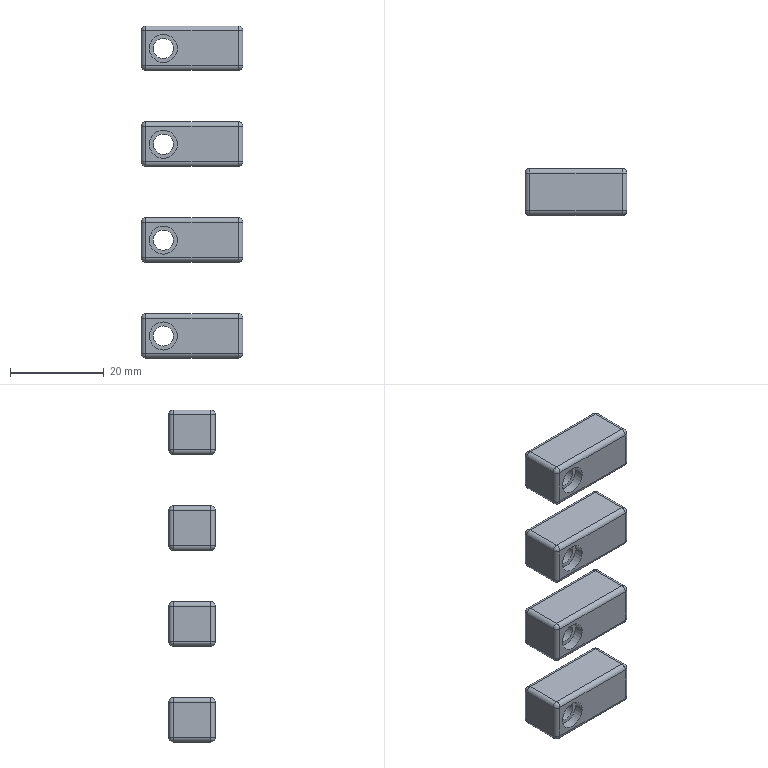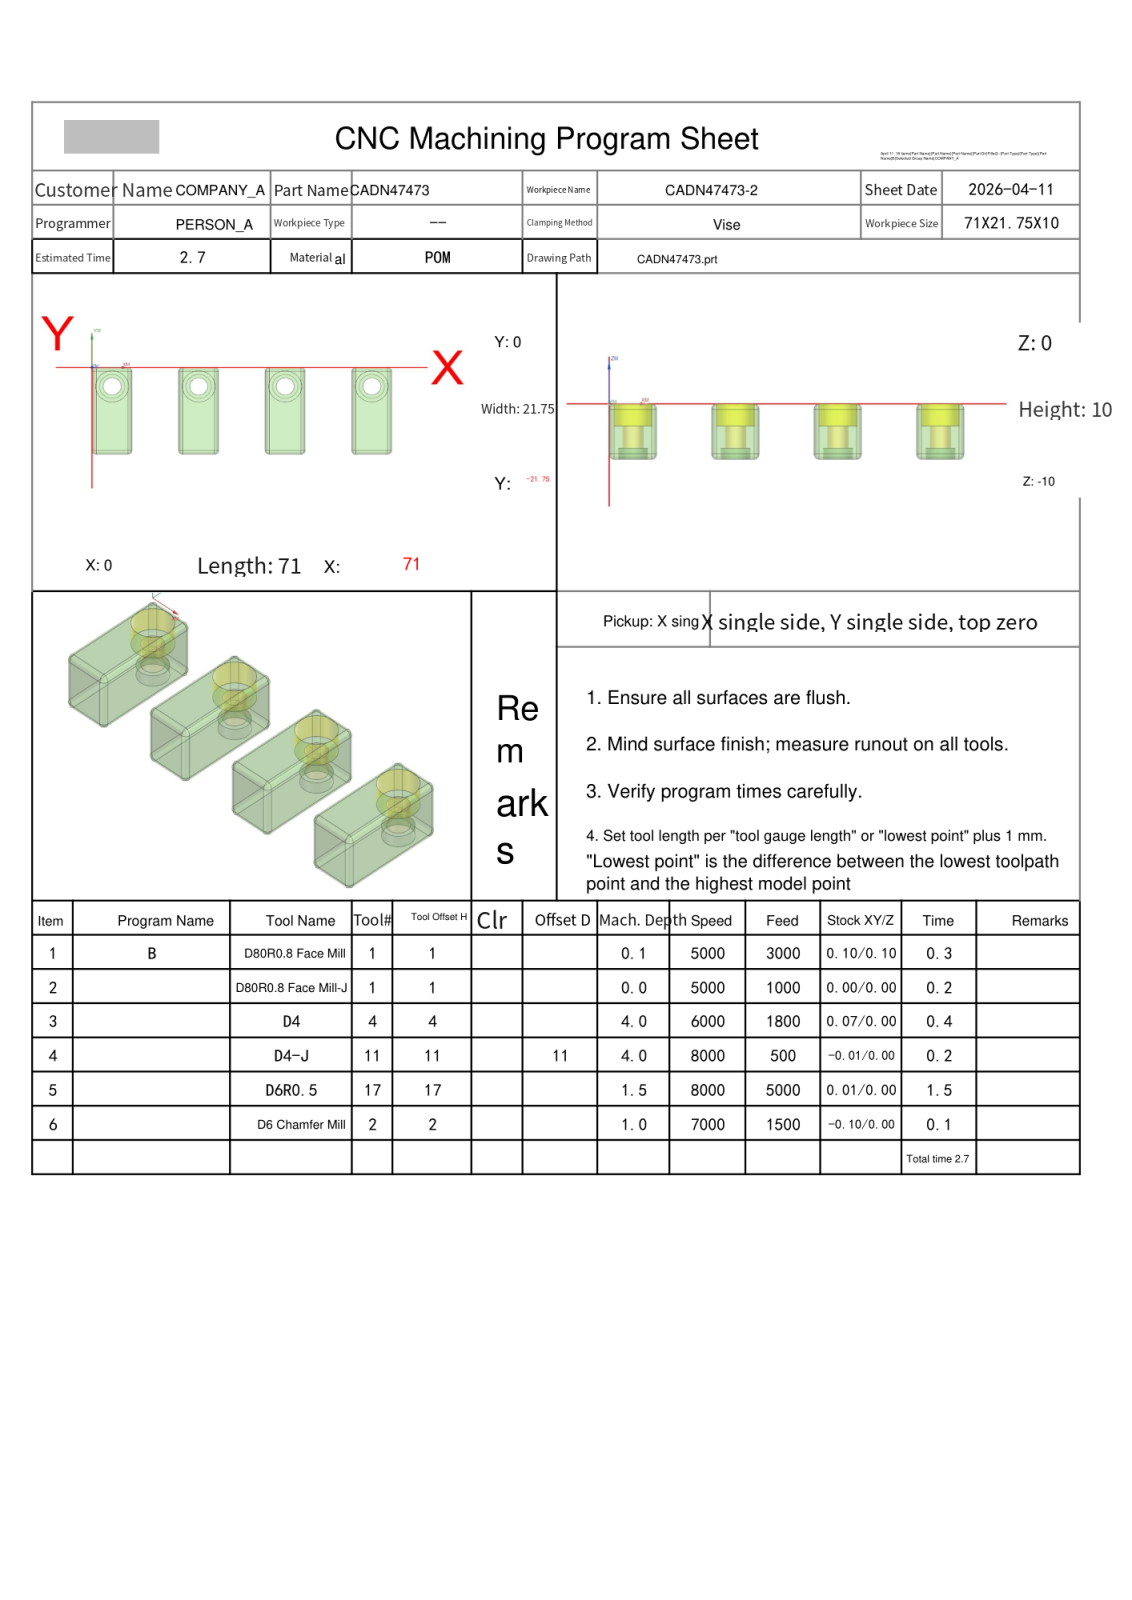NC program | NX | posted by the shop | part box 21.75 x 10 x 71 mm
Lines 14957 to 15118 of 15118:
N6 T02 M06
(D6 Chamfer Mill  D=6. R=0. H=02 ce=-0.10 di=0.00)
G00 G90 G54 X66.939 Y-7.682 M03 S7000
G43 H02 Z20.
M08
Z2.5
G01 X67.274 Y-7.589 Z2.373 F1500.
X67.621 Y-7.445 Z2.237
X67.947 Y-7.259 Z2.1
X68.247 Y-7.033 Z1.963
X68.517 Y-6.772 Z1.827
X68.752 Y-6.479 Z1.69
X68.948 Y-6.159 Z1.553
X69.103 Y-5.817 Z1.417
X69.187 Y-5.562 Z1.319
X69.259 Y-5.241 Z1.199
X69.295 Y-4.914 Z1.08
Y-4.586 Z.96
X69.259 Y-4.259 Z.84
X69.187 Y-3.938 Z.721
X69.103 Y-3.683 Z.623
X68.946 Y-3.338 Z.485
X68.747 Y-3.015 Z.347
X68.509 Y-2.72 Z.209
X68.236 Y-2.457 Z.071
X67.931 Y-2.231 Z-.067
X67.601 Y-2.045 Z-.205
X67.249 Y-1.902 Z-.343
X66.991 Y-1.829 Z-.441
X66.646 Y-1.767 Z-.568
X66.296 Y-1.747 Z-.696
X65.946 Y-1.767 Z-.824
X65.601 Y-1.829 Z-.951
X65.472 Y-1.865 Z-1.
G03 X63.296 Y-4.75 I.824 J-2.885
X66.296 Y-7.75 I3. J0.0
X69.296 Y-4.75 I0.0 J3.
X66.296 Y-1.75 I-3. J0.0
X65.472 Y-1.865 I0.0 J-3.
X65.005 Y-2.042 I.824 J-2.885
G01 Z1.5
G00 Z20.
X46.439 Y-7.682
Z2.5
G01 X46.774 Y-7.589 Z2.373
X47.121 Y-7.445 Z2.237
X47.447 Y-7.259 Z2.1
X47.747 Y-7.033 Z1.963
X48.017 Y-6.772 Z1.827
X48.252 Y-6.479 Z1.69
X48.448 Y-6.159 Z1.553
X48.603 Y-5.817 Z1.417
X48.687 Y-5.562 Z1.319
X48.759 Y-5.241 Z1.199
X48.795 Y-4.914 Z1.08
Y-4.586 Z.96
X48.759 Y-4.259 Z.84
X48.687 Y-3.938 Z.721
X48.603 Y-3.683 Z.623
X48.446 Y-3.338 Z.485
X48.247 Y-3.015 Z.347
X48.009 Y-2.72 Z.209
X47.736 Y-2.457 Z.071
X47.431 Y-2.231 Z-.067
X47.101 Y-2.045 Z-.205
X46.749 Y-1.902 Z-.343
X46.491 Y-1.829 Z-.441
X46.146 Y-1.767 Z-.568
X45.796 Y-1.747 Z-.696
X45.446 Y-1.767 Z-.824
X45.101 Y-1.829 Z-.951
X44.972 Y-1.865 Z-1.
G03 X42.796 Y-4.75 I.824 J-2.885
X45.796 Y-7.75 I3. J0.0
X48.796 Y-4.75 I0.0 J3.
X45.796 Y-1.75 I-3. J0.0
X44.972 Y-1.865 I0.0 J-3.
X44.505 Y-2.042 I.824 J-2.885
G01 Z1.5
G00 Z20.
X25.939 Y-7.682
Z2.5
G01 X26.274 Y-7.589 Z2.373
X26.621 Y-7.445 Z2.237
X26.947 Y-7.259 Z2.1
X27.247 Y-7.033 Z1.963
X27.517 Y-6.772 Z1.827
X27.752 Y-6.479 Z1.69
X27.948 Y-6.159 Z1.553
X28.103 Y-5.817 Z1.417
X28.187 Y-5.562 Z1.319
X28.259 Y-5.241 Z1.199
X28.295 Y-4.914 Z1.08
Y-4.586 Z.96
X28.259 Y-4.259 Z.84
X28.187 Y-3.938 Z.721
X28.103 Y-3.683 Z.623
X27.946 Y-3.338 Z.485
X27.747 Y-3.015 Z.347
X27.509 Y-2.72 Z.209
X27.236 Y-2.457 Z.071
X26.931 Y-2.231 Z-.067
X26.601 Y-2.045 Z-.205
X26.249 Y-1.902 Z-.343
X25.991 Y-1.829 Z-.441
X25.646 Y-1.767 Z-.568
X25.296 Y-1.747 Z-.696
X24.946 Y-1.767 Z-.824
X24.601 Y-1.829 Z-.951
X24.472 Y-1.865 Z-1.
G03 X22.296 Y-4.75 I.824 J-2.885
X25.296 Y-7.75 I3. J0.0
X28.296 Y-4.75 I0.0 J3.
X25.296 Y-1.75 I-3. J0.0
X24.472 Y-1.865 I0.0 J-3.
X24.005 Y-2.042 I.824 J-2.885
G01 Z1.5
G00 Z20.
X5.439 Y-7.682
Z2.5
G01 X5.774 Y-7.589 Z2.373
X6.121 Y-7.445 Z2.237
X6.447 Y-7.259 Z2.1
X6.747 Y-7.033 Z1.963
X7.017 Y-6.772 Z1.827
X7.252 Y-6.479 Z1.69
X7.448 Y-6.159 Z1.553
X7.603 Y-5.817 Z1.417
X7.687 Y-5.562 Z1.319
X7.759 Y-5.241 Z1.199
X7.795 Y-4.914 Z1.08
Y-4.586 Z.96
X7.759 Y-4.259 Z.84
X7.687 Y-3.938 Z.721
X7.603 Y-3.683 Z.623
X7.446 Y-3.338 Z.485
X7.247 Y-3.015 Z.347
X7.009 Y-2.72 Z.209
X6.736 Y-2.457 Z.071
X6.431 Y-2.231 Z-.067
X6.101 Y-2.045 Z-.205
X5.749 Y-1.902 Z-.343
X5.491 Y-1.829 Z-.441
X5.146 Y-1.767 Z-.568
X4.796 Y-1.747 Z-.696
X4.446 Y-1.767 Z-.824
X4.101 Y-1.829 Z-.951
X3.972 Y-1.865 Z-1.
G03 X1.796 Y-4.75 I.824 J-2.885
X4.796 Y-7.75 I3. J0.0
X7.796 Y-4.75 I0.0 J3.
X4.796 Y-1.75 I-3. J0.0
X3.972 Y-1.865 I0.0 J-3.
X3.505 Y-2.042 I.824 J-2.885
G01 Z1.5
G00 Z20.
M05
M09
G91 G28 Z0.0
G91 G28 Y0.0
M30
%